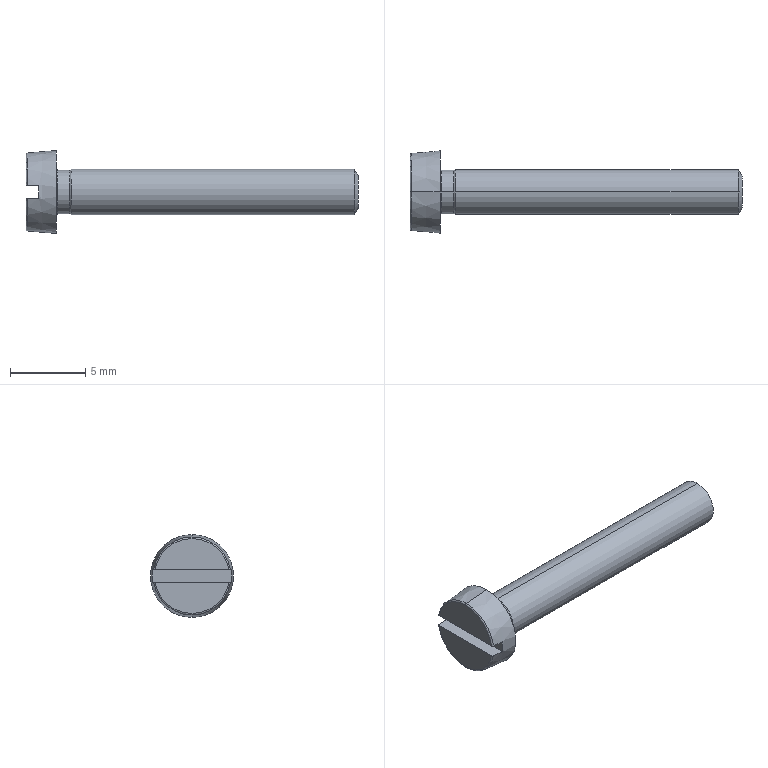Part | SolidWorks | features Cut 1, LPattern 1, RevCut 1, Revolution 1 | 1 solid | 22 faces | box 22 x 5.5 x 5.5 mm | volume 181.48 mm3 | plane 7 | cone 6 | torus 5 | cylinder 4 | commonest cylinder face diameters 2.9 x2 3 x2
STEP:
#1=CARTESIAN_POINT('',(22.,0.,1.067));
#2=VERTEX_POINT('',#1);
#3=CARTESIAN_POINT('',(22.,0.,-1.067));
#4=VERTEX_POINT('',#3);
#5=CARTESIAN_POINT('',(22.,0.,0.));
#6=DIRECTION('',(-1.,0.,0.));
#7=DIRECTION('',(0.,0.,1.));
#8=AXIS2_PLACEMENT_3D('',#5,#6,#7);
#9=CIRCLE('',#8,1.067);
#10=EDGE_CURVE('',#2,#4,#9,.T.);
#11=ORIENTED_EDGE('',*,*,#10,.T.);
#12=CARTESIAN_POINT('',(21.75,0.,-1.5));
#13=VERTEX_POINT('',#12);
#14=CARTESIAN_POINT('',(21.75,0.,-1.5));
#15=DIRECTION('',(-0.5,0.,-0.866));
#16=VECTOR('',#15,1000.);
#17=LINE('',#14,#16);
#18=EDGE_CURVE('',#4,#13,#17,.T.);
#19=ORIENTED_EDGE('',*,*,#18,.T.);
#20=CARTESIAN_POINT('',(21.75,0.,1.5));
#21=VERTEX_POINT('',#20);
#22=CARTESIAN_POINT('',(21.75,0.,0.));
#23=DIRECTION('',(-1.,0.,0.));
#24=DIRECTION('',(0.,0.,1.));
#25=AXIS2_PLACEMENT_3D('',#22,#23,#24);
#26=CIRCLE('',#25,1.5);
#27=EDGE_CURVE('',#21,#13,#26,.T.);
#28=ORIENTED_EDGE('',*,*,#27,.F.);
#29=CARTESIAN_POINT('',(21.75,0.,1.5));
#30=DIRECTION('',(-0.5,0.,0.866));
#31=VECTOR('',#30,1000.);
#32=LINE('',#29,#31);
#33=EDGE_CURVE('',#2,#21,#32,.T.);
#34=ORIENTED_EDGE('',*,*,#33,.F.);
#35=EDGE_LOOP('',(#11,#19,#28,#34));
#36=FACE_OUTER_BOUND('',#35,.T.);
#37=CARTESIAN_POINT('',(21.75,0.,0.));
#38=DIRECTION('',(-1.,0.,0.));
#39=DIRECTION('',(0.,0.,1.));
#40=AXIS2_PLACEMENT_3D('',#37,#38,#39);
#41=CONICAL_SURFACE('',#40,1.5,1.047);
#42=ADVANCED_FACE('',(#36),#41,.T.);
#43=CARTESIAN_POINT('',(2.913,0.,1.45));
#44=VERTEX_POINT('',#43);
#45=CARTESIAN_POINT('',(2.913,0.,-1.45));
#46=VERTEX_POINT('',#45);
#47=CARTESIAN_POINT('',(2.913,0.,0.));
#48=DIRECTION('',(-1.,0.,0.));
#49=DIRECTION('',(0.,0.,1.));
#50=AXIS2_PLACEMENT_3D('',#47,#48,#49);
#51=CIRCLE('',#50,1.45);
#52=EDGE_CURVE('',#44,#46,#51,.T.);
#53=ORIENTED_EDGE('',*,*,#52,.F.);
#54=CARTESIAN_POINT('',(3.,0.,1.5));
#55=VERTEX_POINT('',#54);
#56=CARTESIAN_POINT('',(3.,0.,1.5));
#57=DIRECTION('',(0.866,0.,0.5));
#58=VECTOR('',#57,1000.);
#59=LINE('',#56,#58);
#60=EDGE_CURVE('',#44,#55,#59,.T.);
#61=ORIENTED_EDGE('',*,*,#60,.T.);
#62=CARTESIAN_POINT('',(3.,0.,-1.5));
#63=VERTEX_POINT('',#62);
#64=CARTESIAN_POINT('',(3.,0.,0.));
#65=DIRECTION('',(-1.,0.,0.));
#66=DIRECTION('',(0.,0.,1.));
#67=AXIS2_PLACEMENT_3D('',#64,#65,#66);
#68=CIRCLE('',#67,1.5);
#69=EDGE_CURVE('',#55,#63,#68,.T.);
#70=ORIENTED_EDGE('',*,*,#69,.T.);
#71=CARTESIAN_POINT('',(3.,0.,-1.5));
#72=DIRECTION('',(0.866,0.,-0.5));
#73=VECTOR('',#72,1000.);
#74=LINE('',#71,#73);
#75=EDGE_CURVE('',#46,#63,#74,.T.);
#76=ORIENTED_EDGE('',*,*,#75,.F.);
#77=EDGE_LOOP('',(#53,#61,#70,#76));
#78=FACE_OUTER_BOUND('',#77,.T.);
#79=CARTESIAN_POINT('',(3.,0.,0.));
#80=DIRECTION('',(1.,0.,0.));
#81=DIRECTION('',(0.,0.,-1.));
#82=AXIS2_PLACEMENT_3D('',#79,#80,#81);
#83=CONICAL_SURFACE('',#82,1.5,0.5236);
#84=ADVANCED_FACE('',(#78),#83,.T.);
#85=ORIENTED_EDGE('',*,*,#52,.T.);
#86=CARTESIAN_POINT('',(2.1,0.,-1.45));
#87=VERTEX_POINT('',#86);
#88=CARTESIAN_POINT('',(0.,0.,-1.45));
#89=DIRECTION('',(-1.,0.,0.));
#90=VECTOR('',#89,1000.);
#91=LINE('',#88,#90);
#92=EDGE_CURVE('',#46,#87,#91,.T.);
#93=ORIENTED_EDGE('',*,*,#92,.T.);
#94=CARTESIAN_POINT('',(2.1,0.,1.45));
#95=VERTEX_POINT('',#94);
#96=CARTESIAN_POINT('',(2.1,0.,0.));
#97=DIRECTION('',(-1.,0.,0.));
#98=DIRECTION('',(0.,0.,1.));
#99=AXIS2_PLACEMENT_3D('',#96,#97,#98);
#100=CIRCLE('',#99,1.45);
#101=EDGE_CURVE('',#95,#87,#100,.T.);
#102=ORIENTED_EDGE('',*,*,#101,.F.);
#103=CARTESIAN_POINT('',(0.,0.,1.45));
#104=DIRECTION('',(-1.,0.,0.));
#105=VECTOR('',#104,1000.);
#106=LINE('',#103,#105);
#107=EDGE_CURVE('',#44,#95,#106,.T.);
#108=ORIENTED_EDGE('',*,*,#107,.F.);
#109=EDGE_LOOP('',(#85,#93,#102,#108));
#110=FACE_OUTER_BOUND('',#109,.T.);
#111=CARTESIAN_POINT('',(0.,0.,0.));
#112=DIRECTION('',(-1.,0.,0.));
#113=DIRECTION('',(0.,0.,1.));
#114=AXIS2_PLACEMENT_3D('',#111,#112,#113);
#115=CYLINDRICAL_SURFACE('',#114,1.45);
#116=ADVANCED_FACE('',(#110),#115,.T.);
#117=CARTESIAN_POINT('',(2.,0.,-1.55));
#118=VERTEX_POINT('',#117);
#119=CARTESIAN_POINT('',(2.,0.,1.55));
#120=VERTEX_POINT('',#119);
#121=CARTESIAN_POINT('',(2.,0.,0.));
#122=DIRECTION('',(-1.,0.,0.));
#123=DIRECTION('',(0.,0.,1.));
#124=AXIS2_PLACEMENT_3D('',#121,#122,#123);
#125=CIRCLE('',#124,1.55);
#126=EDGE_CURVE('',#118,#120,#125,.T.);
#127=ORIENTED_EDGE('',*,*,#126,.F.);
#128=CARTESIAN_POINT('',(2.1,0.,-1.55));
#129=DIRECTION('',(0.,1.,0.));
#130=DIRECTION('',(0.,0.,1.));
#131=AXIS2_PLACEMENT_3D('',#128,#129,#130);
#132=CIRCLE('',#131,0.1);
#133=EDGE_CURVE('',#118,#87,#132,.T.);
#134=ORIENTED_EDGE('',*,*,#133,.T.);
#135=CARTESIAN_POINT('',(2.1,0.,0.));
#136=DIRECTION('',(-1.,0.,0.));
#137=DIRECTION('',(0.,0.,1.));
#138=AXIS2_PLACEMENT_3D('',#135,#136,#137);
#139=CIRCLE('',#138,1.45);
#140=EDGE_CURVE('',#87,#95,#139,.T.);
#141=ORIENTED_EDGE('',*,*,#140,.T.);
#142=CARTESIAN_POINT('',(2.1,0.,1.55));
#143=DIRECTION('',(0.,-1.,0.));
#144=DIRECTION('',(0.,0.,-1.));
#145=AXIS2_PLACEMENT_3D('',#142,#143,#144);
#146=CIRCLE('',#145,0.1);
#147=EDGE_CURVE('',#120,#95,#146,.T.);
#148=ORIENTED_EDGE('',*,*,#147,.F.);
#149=EDGE_LOOP('',(#127,#134,#141,#148));
#150=FACE_OUTER_BOUND('',#149,.T.);
#151=CARTESIAN_POINT('',(2.1,0.,0.));
#152=DIRECTION('',(-1.,0.,0.));
#153=DIRECTION('',(0.,0.,1.));
#154=AXIS2_PLACEMENT_3D('',#151,#152,#153);
#155=TOROIDAL_SURFACE('',#154,1.55,0.1);
#156=ADVANCED_FACE('',(#150),#155,.F.);
#157=CARTESIAN_POINT('',(0.09128,0.,2.583));
#158=VERTEX_POINT('',#157);
#159=CARTESIAN_POINT('',(0.09128,2.552,0.4));
#160=VERTEX_POINT('',#159);
#161=CARTESIAN_POINT('',(0.09128,0.,0.));
#162=DIRECTION('',(-1.,0.,0.));
#163=DIRECTION('',(0.,0.,1.));
#164=AXIS2_PLACEMENT_3D('',#161,#162,#163);
#165=CIRCLE('',#164,2.583);
#166=EDGE_CURVE('',#158,#160,#165,.T.);
#167=ORIENTED_EDGE('',*,*,#166,.F.);
#168=CARTESIAN_POINT('',(2.,0.,2.75));
#169=VERTEX_POINT('',#168);
#170=CARTESIAN_POINT('',(2.,0.,2.75));
#171=DIRECTION('',(0.9962,0.,0.08716));
#172=VECTOR('',#171,1000.);
#173=LINE('',#170,#172);
#174=EDGE_CURVE('',#158,#169,#173,.T.);
#175=ORIENTED_EDGE('',*,*,#174,.T.);
#176=CARTESIAN_POINT('',(2.,0.,-2.75));
#177=VERTEX_POINT('',#176);
#178=CARTESIAN_POINT('',(2.,0.,0.));
#179=DIRECTION('',(-1.,0.,0.));
#180=DIRECTION('',(0.,0.,1.));
#181=AXIS2_PLACEMENT_3D('',#178,#179,#180);
#182=CIRCLE('',#181,2.75);
#183=EDGE_CURVE('',#169,#177,#182,.T.);
#184=ORIENTED_EDGE('',*,*,#183,.T.);
#185=CARTESIAN_POINT('',(0.09128,0.,-2.583));
#186=VERTEX_POINT('',#185);
#187=CARTESIAN_POINT('',(2.,0.,-2.75));
#188=DIRECTION('',(0.9962,0.,-0.08716));
#189=VECTOR('',#188,1000.);
#190=LINE('',#187,#189);
#191=EDGE_CURVE('',#186,#177,#190,.T.);
#192=ORIENTED_EDGE('',*,*,#191,.F.);
#193=CARTESIAN_POINT('',(0.09128,2.552,-0.4));
#194=VERTEX_POINT('',#193);
#195=CARTESIAN_POINT('',(0.09128,0.,0.));
#196=DIRECTION('',(-1.,0.,0.));
#197=DIRECTION('',(0.,0.,1.));
#198=AXIS2_PLACEMENT_3D('',#195,#196,#197);
#199=CIRCLE('',#198,2.583);
#200=EDGE_CURVE('',#194,#186,#199,.T.);
#201=ORIENTED_EDGE('',*,*,#200,.F.);
#202=CARTESIAN_POINT('',(0.85,2.619,-0.4));
#203=VERTEX_POINT('',#202);
#204=CARTESIAN_POINT('',(0.09128,2.552,-0.4));
#205=CARTESIAN_POINT('',(0.2017,2.562,-0.4));
#206=CARTESIAN_POINT('',(0.3121,2.571,-0.4));
#207=CARTESIAN_POINT('',(0.4225,2.581,-0.4));
#208=CARTESIAN_POINT('',(0.565,2.594,-0.4));
#209=CARTESIAN_POINT('',(0.7075,2.606,-0.4));
#210=CARTESIAN_POINT('',(0.85,2.619,-0.4));
#211=B_SPLINE_CURVE_WITH_KNOTS('',3,(#204,#205,#206,#207,#208,#209,#210),.UNSPECIFIED.,.F.,.F.,(4,3,4),(0.004473,0.004805,0.005234),.UNSPECIFIED.);
#212=EDGE_CURVE('',#194,#203,#211,.T.);
#213=ORIENTED_EDGE('',*,*,#212,.T.);
#214=CARTESIAN_POINT('',(0.85,2.619,0.4));
#215=VERTEX_POINT('',#214);
#216=CARTESIAN_POINT('',(0.85,0.,0.));
#217=DIRECTION('',(-1.,0.,0.));
#218=DIRECTION('',(0.,-1.,0.));
#219=AXIS2_PLACEMENT_3D('',#216,#217,#218);
#220=CIRCLE('',#219,2.649);
#221=EDGE_CURVE('',#215,#203,#220,.T.);
#222=ORIENTED_EDGE('',*,*,#221,.F.);
#223=CARTESIAN_POINT('',(0.85,2.619,0.4));
#224=CARTESIAN_POINT('',(0.7075,2.606,0.4));
#225=CARTESIAN_POINT('',(0.565,2.594,0.4));
#226=CARTESIAN_POINT('',(0.4225,2.581,0.4));
#227=CARTESIAN_POINT('',(0.3121,2.571,0.4));
#228=CARTESIAN_POINT('',(0.2017,2.562,0.4));
#229=CARTESIAN_POINT('',(0.09128,2.552,0.4));
#230=B_SPLINE_CURVE_WITH_KNOTS('',3,(#223,#224,#225,#226,#227,#228,#229),.UNSPECIFIED.,.F.,.F.,(4,3,4),(0.004376,0.004805,0.005138),.UNSPECIFIED.);
#231=EDGE_CURVE('',#215,#160,#230,.T.);
#232=ORIENTED_EDGE('',*,*,#231,.T.);
#233=EDGE_LOOP('',(#167,#175,#184,#192,#201,#213,#222,#232));
#234=FACE_OUTER_BOUND('',#233,.T.);
#235=CARTESIAN_POINT('',(2.,0.,0.));
#236=DIRECTION('',(1.,0.,0.));
#237=DIRECTION('',(0.,0.,-1.));
#238=AXIS2_PLACEMENT_3D('',#235,#236,#237);
#239=CONICAL_SURFACE('',#238,2.75,0.08727);
#240=ADVANCED_FACE('',(#234),#239,.T.);
#241=CARTESIAN_POINT('',(0.09128,-2.552,0.4));
#242=VERTEX_POINT('',#241);
#243=CARTESIAN_POINT('',(0.09128,0.,0.));
#244=DIRECTION('',(-1.,0.,0.));
#245=DIRECTION('',(0.,0.,1.));
#246=AXIS2_PLACEMENT_3D('',#243,#244,#245);
#247=CIRCLE('',#246,2.583);
#248=EDGE_CURVE('',#242,#158,#247,.T.);
#249=ORIENTED_EDGE('',*,*,#248,.T.);
#250=CARTESIAN_POINT('',(0.,0.,2.483));
#251=VERTEX_POINT('',#250);
#252=CARTESIAN_POINT('',(0.1,0.,2.483));
#253=DIRECTION('',(0.,-1.,0.));
#254=DIRECTION('',(0.,0.,-1.));
#255=AXIS2_PLACEMENT_3D('',#252,#253,#254);
#256=CIRCLE('',#255,0.1);
#257=EDGE_CURVE('',#158,#251,#256,.T.);
#258=ORIENTED_EDGE('',*,*,#257,.T.);
#259=CARTESIAN_POINT('',(0.,-2.451,0.4));
#260=VERTEX_POINT('',#259);
#261=CARTESIAN_POINT('',(0.,0.,0.));
#262=DIRECTION('',(-1.,0.,0.));
#263=DIRECTION('',(0.,0.,1.));
#264=AXIS2_PLACEMENT_3D('',#261,#262,#263);
#265=CIRCLE('',#264,2.483);
#266=EDGE_CURVE('',#260,#251,#265,.T.);
#267=ORIENTED_EDGE('',*,*,#266,.F.);
#268=CARTESIAN_POINT('',(0.,-2.451,0.4));
#269=CARTESIAN_POINT('',(0.,-2.458,0.4));
#270=CARTESIAN_POINT('',(0.0008068,-2.466,0.4));
#271=CARTESIAN_POINT('',(0.002394,-2.473,0.4));
#272=CARTESIAN_POINT('',(0.004862,-2.484,0.4));
#273=CARTESIAN_POINT('',(0.009305,-2.495,0.4));
#274=CARTESIAN_POINT('',(0.01537,-2.505,0.4));
#275=CARTESIAN_POINT('',(0.01925,-2.511,0.4));
#276=CARTESIAN_POINT('',(0.02385,-2.517,0.4));
#277=CARTESIAN_POINT('',(0.02899,-2.522,0.4));
#278=CARTESIAN_POINT('',(0.03681,-2.53,0.4));
#279=CARTESIAN_POINT('',(0.04609,-2.537,0.4));
#280=CARTESIAN_POINT('',(0.0561,-2.542,0.4));
#281=CARTESIAN_POINT('',(0.06611,-2.547,0.4));
#282=CARTESIAN_POINT('',(0.07712,-2.55,0.4));
#283=CARTESIAN_POINT('',(0.0882,-2.552,0.4));
#284=CARTESIAN_POINT('',(0.08923,-2.552,0.4));
#285=CARTESIAN_POINT('',(0.09026,-2.552,0.4));
#286=CARTESIAN_POINT('',(0.09128,-2.552,0.4));
#287=B_SPLINE_CURVE_WITH_KNOTS('',3,(#268,#269,#270,#271,#272,#273,#274,#275,#276,#277,#278,#279,#280,#281,#282,#283,#284,#285,#286),.UNSPECIFIED.,.F.,.F.,(4,3,3,3,3,3,4),(0.0005509,0.0005731,0.0006075,0.0006294,0.0006629,0.0006964,0.0006995),.UNSPECIFIED.);
#288=EDGE_CURVE('',#260,#242,#287,.T.);
#289=ORIENTED_EDGE('',*,*,#288,.T.);
#290=EDGE_LOOP('',(#249,#258,#267,#289));
#291=FACE_OUTER_BOUND('',#290,.T.);
#292=CARTESIAN_POINT('',(0.1,0.,0.));
#293=DIRECTION('',(-1.,0.,0.));
#294=DIRECTION('',(0.,0.,1.));
#295=AXIS2_PLACEMENT_3D('',#292,#293,#294);
#296=TOROIDAL_SURFACE('',#295,2.483,0.1);
#297=ADVANCED_FACE('',(#291),#296,.T.);
#298=ORIENTED_EDGE('',*,*,#27,.T.);
#299=CARTESIAN_POINT('',(0.,0.,-1.5));
#300=DIRECTION('',(-1.,0.,0.));
#301=VECTOR('',#300,1000.);
#302=LINE('',#299,#301);
#303=EDGE_CURVE('',#13,#63,#302,.T.);
#304=ORIENTED_EDGE('',*,*,#303,.T.);
#305=ORIENTED_EDGE('',*,*,#69,.F.);
#306=CARTESIAN_POINT('',(0.,0.,1.5));
#307=DIRECTION('',(-1.,0.,0.));
#308=VECTOR('',#307,1000.);
#309=LINE('',#306,#308);
#310=EDGE_CURVE('',#21,#55,#309,.T.);
#311=ORIENTED_EDGE('',*,*,#310,.F.);
#312=EDGE_LOOP('',(#298,#304,#305,#311));
#313=FACE_OUTER_BOUND('',#312,.T.);
#314=CARTESIAN_POINT('',(0.,0.,0.));
#315=DIRECTION('',(-1.,0.,0.));
#316=DIRECTION('',(0.,0.,1.));
#317=AXIS2_PLACEMENT_3D('',#314,#315,#316);
#318=CYLINDRICAL_SURFACE('',#317,1.5);
#319=ADVANCED_FACE('',(#313),#318,.T.);
#320=ORIENTED_EDGE('',*,*,#303,.F.);
#321=CARTESIAN_POINT('',(21.75,0.,0.));
#322=DIRECTION('',(-1.,0.,0.));
#323=DIRECTION('',(0.,0.,1.));
#324=AXIS2_PLACEMENT_3D('',#321,#322,#323);
#325=CIRCLE('',#324,1.5);
#326=EDGE_CURVE('',#13,#21,#325,.T.);
#327=ORIENTED_EDGE('',*,*,#326,.T.);
#328=ORIENTED_EDGE('',*,*,#310,.T.);
#329=CARTESIAN_POINT('',(3.,0.,0.));
#330=DIRECTION('',(-1.,0.,0.));
#331=DIRECTION('',(0.,0.,1.));
#332=AXIS2_PLACEMENT_3D('',#329,#330,#331);
#333=CIRCLE('',#332,1.5);
#334=EDGE_CURVE('',#63,#55,#333,.T.);
#335=ORIENTED_EDGE('',*,*,#334,.F.);
#336=EDGE_LOOP('',(#320,#327,#328,#335));
#337=FACE_OUTER_BOUND('',#336,.T.);
#338=CARTESIAN_POINT('',(0.,0.,0.));
#339=DIRECTION('',(-1.,0.,0.));
#340=DIRECTION('',(0.,0.,1.));
#341=AXIS2_PLACEMENT_3D('',#338,#339,#340);
#342=CYLINDRICAL_SURFACE('',#341,1.5);
#343=ADVANCED_FACE('',(#337),#342,.T.);
#344=ORIENTED_EDGE('',*,*,#266,.T.);
#345=CARTESIAN_POINT('',(0.,2.451,0.4));
#346=VERTEX_POINT('',#345);
#347=CARTESIAN_POINT('',(0.,0.,0.));
#348=DIRECTION('',(-1.,0.,0.));
#349=DIRECTION('',(0.,0.,1.));
#350=AXIS2_PLACEMENT_3D('',#347,#348,#349);
#351=CIRCLE('',#350,2.483);
#352=EDGE_CURVE('',#251,#346,#351,.T.);
#353=ORIENTED_EDGE('',*,*,#352,.T.);
#354=CARTESIAN_POINT('',(0.,2.721,0.4));
#355=DIRECTION('',(0.,1.,0.));
#356=VECTOR('',#355,1000.);
#357=LINE('',#354,#356);
#358=EDGE_CURVE('',#260,#346,#357,.T.);
#359=ORIENTED_EDGE('',*,*,#358,.F.);
#360=EDGE_LOOP('',(#344,#353,#359));
#361=FACE_OUTER_BOUND('',#360,.T.);
#362=CARTESIAN_POINT('',(0.,0.,0.));
#363=DIRECTION('',(1.,0.,0.));
#364=DIRECTION('',(0.,0.,-1.));
#365=AXIS2_PLACEMENT_3D('',#362,#363,#364);
#366=PLANE('',#365);
#367=ADVANCED_FACE('',(#361),#366,.F.);
#368=ORIENTED_EDGE('',*,*,#257,.F.);
#369=ORIENTED_EDGE('',*,*,#166,.T.);
#370=CARTESIAN_POINT('',(0.09128,2.552,0.4));
#371=CARTESIAN_POINT('',(0.08707,2.551,0.4));
#372=CARTESIAN_POINT('',(0.08288,2.551,0.4));
#373=CARTESIAN_POINT('',(0.07875,2.55,0.4));
#374=CARTESIAN_POINT('',(0.06795,2.548,0.4));
#375=CARTESIAN_POINT('',(0.05741,2.543,0.4));
#376=CARTESIAN_POINT('',(0.048,2.537,0.4));
#377=CARTESIAN_POINT('',(0.03854,2.532,0.4));
#378=CARTESIAN_POINT('',(0.02995,2.524,0.4));
#379=CARTESIAN_POINT('',(0.02293,2.516,0.4));
#380=CARTESIAN_POINT('',(0.01583,2.507,0.4));
#381=CARTESIAN_POINT('',(0.01012,2.497,0.4));
#382=CARTESIAN_POINT('',(0.006257,2.486,0.4));
#383=CARTESIAN_POINT('',(0.002345,2.476,0.4));
#384=CARTESIAN_POINT('',(0.0002101,2.464,0.4));
#385=CARTESIAN_POINT('',(0.00001512,2.453,0.4));
#386=CARTESIAN_POINT('',(0.00000504,2.452,0.4));
#387=CARTESIAN_POINT('',(0.,2.452,0.4));
#388=CARTESIAN_POINT('',(0.,2.451,0.4));
#389=B_SPLINE_CURVE_WITH_KNOTS('',3,(#370,#371,#372,#373,#374,#375,#376,#377,#378,#379,#380,#381,#382,#383,#384,#385,#386,#387,#388),.UNSPECIFIED.,.F.,.F.,(4,3,3,3,3,3,4),(0.0003918,0.0004044,0.0004376,0.0004709,0.0005046,0.0005387,0.0005404),.UNSPECIFIED.);
#390=EDGE_CURVE('',#160,#346,#389,.T.);
#391=ORIENTED_EDGE('',*,*,#390,.T.);
#392=ORIENTED_EDGE('',*,*,#352,.F.);
#393=EDGE_LOOP('',(#368,#369,#391,#392));
#394=FACE_OUTER_BOUND('',#393,.T.);
#395=CARTESIAN_POINT('',(0.1,0.,0.));
#396=DIRECTION('',(-1.,0.,0.));
#397=DIRECTION('',(0.,0.,1.));
#398=AXIS2_PLACEMENT_3D('',#395,#396,#397);
#399=TOROIDAL_SURFACE('',#398,2.483,0.1);
#400=ADVANCED_FACE('',(#394),#399,.T.);
#401=CARTESIAN_POINT('',(0.,2.451,-0.4));
#402=VERTEX_POINT('',#401);
#403=CARTESIAN_POINT('',(0.,-2.451,-0.4));
#404=VERTEX_POINT('',#403);
#405=CARTESIAN_POINT('',(0.,0.,0.));
#406=DIRECTION('',(-1.,0.,0.));
#407=DIRECTION('',(0.,0.,1.));
#408=AXIS2_PLACEMENT_3D('',#405,#406,#407);
#409=CIRCLE('',#408,2.483);
#410=EDGE_CURVE('',#402,#404,#409,.T.);
#411=ORIENTED_EDGE('',*,*,#410,.T.);
#412=CARTESIAN_POINT('',(0.,2.721,-0.4));
#413=DIRECTION('',(0.,-1.,0.));
#414=VECTOR('',#413,1000.);
#415=LINE('',#412,#414);
#416=EDGE_CURVE('',#402,#404,#415,.T.);
#417=ORIENTED_EDGE('',*,*,#416,.F.);
#418=EDGE_LOOP('',(#411,#417));
#419=FACE_OUTER_BOUND('',#418,.T.);
#420=CARTESIAN_POINT('',(0.,0.,0.));
#421=DIRECTION('',(1.,0.,0.));
#422=DIRECTION('',(0.,0.,-1.));
#423=AXIS2_PLACEMENT_3D('',#420,#421,#422);
#424=PLANE('',#423);
#425=ADVANCED_FACE('',(#419),#424,.F.);
#426=ORIENTED_EDGE('',*,*,#200,.T.);
#427=CARTESIAN_POINT('',(0.09128,-2.552,-0.4));
#428=VERTEX_POINT('',#427);
#429=CARTESIAN_POINT('',(0.09128,0.,0.));
#430=DIRECTION('',(-1.,0.,0.));
#431=DIRECTION('',(0.,0.,1.));
#432=AXIS2_PLACEMENT_3D('',#429,#430,#431);
#433=CIRCLE('',#432,2.583);
#434=EDGE_CURVE('',#186,#428,#433,.T.);
#435=ORIENTED_EDGE('',*,*,#434,.T.);
#436=CARTESIAN_POINT('',(0.09128,-2.552,-0.4));
#437=CARTESIAN_POINT('',(0.08571,-2.551,-0.4));
#438=CARTESIAN_POINT('',(0.08015,-2.55,-0.4));
#439=CARTESIAN_POINT('',(0.07474,-2.549,-0.4));
#440=CARTESIAN_POINT('',(0.06404,-2.546,-0.4));
#441=CARTESIAN_POINT('',(0.05369,-2.541,-0.4));
#442=CARTESIAN_POINT('',(0.04452,-2.535,-0.4));
#443=CARTESIAN_POINT('',(0.03893,-2.531,-0.4));
#444=CARTESIAN_POINT('',(0.03371,-2.527,-0.4));
#445=CARTESIAN_POINT('',(0.02899,-2.522,-0.4));
#446=CARTESIAN_POINT('',(0.02104,-2.514,-0.4));
#447=CARTESIAN_POINT('',(0.0144,-2.505,-0.4));
#448=CARTESIAN_POINT('',(0.009591,-2.494,-0.4));
#449=CARTESIAN_POINT('',(0.004787,-2.484,-0.4));
#450=CARTESIAN_POINT('',(0.001687,-2.473,-0.4));
#451=CARTESIAN_POINT('',(0.0005321,-2.461,-0.4));
#452=CARTESIAN_POINT('',(0.0001778,-2.458,-0.4));
#453=CARTESIAN_POINT('',(0.,-2.454,-0.4));
#454=CARTESIAN_POINT('',(0.,-2.451,-0.4));
#455=B_SPLINE_CURVE_WITH_KNOTS('',3,(#436,#437,#438,#439,#440,#441,#442,#443,#444,#445,#446,#447,#448,#449,#450,#451,#452,#453,#454),.UNSPECIFIED.,.F.,.F.,(4,3,3,3,3,3,4),(0.0005594,0.0005761,0.0006093,0.0006293,0.0006634,0.0006975,0.0007078),.UNSPECIFIED.);
#456=EDGE_CURVE('',#428,#404,#455,.T.);
#457=ORIENTED_EDGE('',*,*,#456,.T.);
#458=ORIENTED_EDGE('',*,*,#410,.F.);
#459=CARTESIAN_POINT('',(0.,2.451,-0.4));
#460=CARTESIAN_POINT('',(0.,2.455,-0.4));
#461=CARTESIAN_POINT('',(0.000287,2.46,-0.4));
#462=CARTESIAN_POINT('',(0.0008577,2.464,-0.4));
#463=CARTESIAN_POINT('',(0.00234,2.476,-0.4));
#464=CARTESIAN_POINT('',(0.005811,2.487,-0.4));
#465=CARTESIAN_POINT('',(0.011,2.497,-0.4));
#466=CARTESIAN_POINT('',(0.01616,2.507,-0.4));
#467=CARTESIAN_POINT('',(0.02317,2.517,-0.4));
#468=CARTESIAN_POINT('',(0.03145,2.525,-0.4));
#469=CARTESIAN_POINT('',(0.03965,2.533,-0.4));
#470=CARTESIAN_POINT('',(0.04932,2.539,-0.4));
#471=CARTESIAN_POINT('',(0.05966,2.544,-0.4));
#472=CARTESIAN_POINT('',(0.0696,2.548,-0.4));
#473=CARTESIAN_POINT('',(0.08043,2.551,-0.4));
#474=CARTESIAN_POINT('',(0.09128,2.552,-0.4));
#475=B_SPLINE_CURVE_WITH_KNOTS('',3,(#459,#460,#461,#462,#463,#464,#465,#466,#467,#468,#469,#470,#471,#472,#473,#474),.UNSPECIFIED.,.F.,.F.,(4,3,3,3,3,4),(0.00008915,0.0001023,0.0001368,0.0001712,0.0002051,0.0002378),.UNSPECIFIED.);
#476=EDGE_CURVE('',#402,#194,#475,.T.);
#477=ORIENTED_EDGE('',*,*,#476,.T.);
#478=EDGE_LOOP('',(#426,#435,#457,#458,#477));
#479=FACE_OUTER_BOUND('',#478,.T.);
#480=CARTESIAN_POINT('',(0.1,0.,0.));
#481=DIRECTION('',(-1.,0.,0.));
#482=DIRECTION('',(0.,0.,1.));
#483=AXIS2_PLACEMENT_3D('',#480,#481,#482);
#484=TOROIDAL_SURFACE('',#483,2.483,0.1);
#485=ADVANCED_FACE('',(#479),#484,.T.);
#486=ORIENTED_EDGE('',*,*,#174,.F.);
#487=ORIENTED_EDGE('',*,*,#248,.F.);
#488=CARTESIAN_POINT('',(0.85,-2.619,0.4));
#489=VERTEX_POINT('',#488);
#490=CARTESIAN_POINT('',(0.09128,-2.552,0.4));
#491=CARTESIAN_POINT('',(0.2017,-2.562,0.4));
#492=CARTESIAN_POINT('',(0.3121,-2.571,0.4));
#493=CARTESIAN_POINT('',(0.4225,-2.581,0.4));
#494=CARTESIAN_POINT('',(0.565,-2.594,0.4));
#495=CARTESIAN_POINT('',(0.7075,-2.606,0.4));
#496=CARTESIAN_POINT('',(0.85,-2.619,0.4));
#497=B_SPLINE_CURVE_WITH_KNOTS('',3,(#490,#491,#492,#493,#494,#495,#496),.UNSPECIFIED.,.F.,.F.,(4,3,4),(0.004473,0.004805,0.005234),.UNSPECIFIED.);
#498=EDGE_CURVE('',#242,#489,#497,.T.);
#499=ORIENTED_EDGE('',*,*,#498,.T.);
#500=CARTESIAN_POINT('',(0.85,-2.619,-0.4));
#501=VERTEX_POINT('',#500);
#502=CARTESIAN_POINT('',(0.85,0.,0.));
#503=DIRECTION('',(-1.,0.,0.));
#504=DIRECTION('',(0.,-1.,0.));
#505=AXIS2_PLACEMENT_3D('',#502,#503,#504);
#506=CIRCLE('',#505,2.649);
#507=EDGE_CURVE('',#501,#489,#506,.T.);
#508=ORIENTED_EDGE('',*,*,#507,.F.);
#509=CARTESIAN_POINT('',(0.85,-2.619,-0.4));
#510=CARTESIAN_POINT('',(0.7075,-2.606,-0.4));
#511=CARTESIAN_POINT('',(0.565,-2.594,-0.4));
#512=CARTESIAN_POINT('',(0.4225,-2.581,-0.4));
#513=CARTESIAN_POINT('',(0.3121,-2.571,-0.4));
#514=CARTESIAN_POINT('',(0.2017,-2.562,-0.4));
#515=CARTESIAN_POINT('',(0.09128,-2.552,-0.4));
#516=B_SPLINE_CURVE_WITH_KNOTS('',3,(#509,#510,#511,#512,#513,#514,#515),.UNSPECIFIED.,.F.,.F.,(4,3,4),(0.004376,0.004805,0.005138),.UNSPECIFIED.);
#517=EDGE_CURVE('',#501,#428,#516,.T.);
#518=ORIENTED_EDGE('',*,*,#517,.T.);
#519=ORIENTED_EDGE('',*,*,#434,.F.);
#520=ORIENTED_EDGE('',*,*,#191,.T.);
#521=CARTESIAN_POINT('',(2.,0.,0.));
#522=DIRECTION('',(-1.,0.,0.));
#523=DIRECTION('',(0.,0.,1.));
#524=AXIS2_PLACEMENT_3D('',#521,#522,#523);
#525=CIRCLE('',#524,2.75);
#526=EDGE_CURVE('',#177,#169,#525,.T.);
#527=ORIENTED_EDGE('',*,*,#526,.T.);
#528=EDGE_LOOP('',(#486,#487,#499,#508,#518,#519,#520,#527));
#529=FACE_OUTER_BOUND('',#528,.T.);
#530=CARTESIAN_POINT('',(2.,0.,0.));
#531=DIRECTION('',(1.,0.,0.));
#532=DIRECTION('',(0.,0.,-1.));
#533=AXIS2_PLACEMENT_3D('',#530,#531,#532);
#534=CONICAL_SURFACE('',#533,2.75,0.08727);
#535=ADVANCED_FACE('',(#529),#534,.T.);
#536=ORIENTED_EDGE('',*,*,#526,.F.);
#537=ORIENTED_EDGE('',*,*,#183,.F.);
#538=EDGE_LOOP('',(#536,#537));
#539=FACE_OUTER_BOUND('',#538,.T.);
#540=CARTESIAN_POINT('',(2.,0.,0.));
#541=DIRECTION('',(-1.,0.,0.));
#542=DIRECTION('',(0.,0.,1.));
#543=AXIS2_PLACEMENT_3D('',#540,#541,#542);
#544=CIRCLE('',#543,1.55);
#545=EDGE_CURVE('',#120,#118,#544,.T.);
#546=ORIENTED_EDGE('',*,*,#545,.T.);
#547=ORIENTED_EDGE('',*,*,#126,.T.);
#548=EDGE_LOOP('',(#546,#547));
#549=FACE_BOUND('',#548,.T.);
#550=CARTESIAN_POINT('',(2.,2.75,0.));
#551=DIRECTION('',(-1.,0.,0.));
#552=DIRECTION('',(0.,0.,1.));
#553=AXIS2_PLACEMENT_3D('',#550,#551,#552);
#554=PLANE('',#553);
#555=ADVANCED_FACE('',(#539,#549),#554,.F.);
#556=ORIENTED_EDGE('',*,*,#133,.F.);
#557=ORIENTED_EDGE('',*,*,#545,.F.);
#558=ORIENTED_EDGE('',*,*,#147,.T.);
#559=ORIENTED_EDGE('',*,*,#101,.T.);
#560=EDGE_LOOP('',(#556,#557,#558,#559));
#561=FACE_OUTER_BOUND('',#560,.T.);
#562=CARTESIAN_POINT('',(2.1,0.,0.));
#563=DIRECTION('',(-1.,0.,0.));
#564=DIRECTION('',(0.,0.,1.));
#565=AXIS2_PLACEMENT_3D('',#562,#563,#564);
#566=TOROIDAL_SURFACE('',#565,1.55,0.1);
#567=ADVANCED_FACE('',(#561),#566,.F.);
#568=ORIENTED_EDGE('',*,*,#92,.F.);
#569=CARTESIAN_POINT('',(2.913,0.,0.));
#570=DIRECTION('',(-1.,0.,0.));
#571=DIRECTION('',(0.,0.,1.));
#572=AXIS2_PLACEMENT_3D('',#569,#570,#571);
#573=CIRCLE('',#572,1.45);
#574=EDGE_CURVE('',#46,#44,#573,.T.);
#575=ORIENTED_EDGE('',*,*,#574,.T.);
#576=ORIENTED_EDGE('',*,*,#107,.T.);
#577=ORIENTED_EDGE('',*,*,#140,.F.);
#578=EDGE_LOOP('',(#568,#575,#576,#577));
#579=FACE_OUTER_BOUND('',#578,.T.);
#580=CARTESIAN_POINT('',(0.,0.,0.));
#581=DIRECTION('',(-1.,0.,0.));
#582=DIRECTION('',(0.,0.,1.));
#583=AXIS2_PLACEMENT_3D('',#580,#581,#582);
#584=CYLINDRICAL_SURFACE('',#583,1.45);
#585=ADVANCED_FACE('',(#579),#584,.T.);
#586=ORIENTED_EDGE('',*,*,#60,.F.);
#587=ORIENTED_EDGE('',*,*,#574,.F.);
#588=ORIENTED_EDGE('',*,*,#75,.T.);
#589=ORIENTED_EDGE('',*,*,#334,.T.);
#590=EDGE_LOOP('',(#586,#587,#588,#589));
#591=FACE_OUTER_BOUND('',#590,.T.);
#592=CARTESIAN_POINT('',(3.,0.,0.));
#593=DIRECTION('',(1.,0.,0.));
#594=DIRECTION('',(0.,0.,-1.));
#595=AXIS2_PLACEMENT_3D('',#592,#593,#594);
#596=CONICAL_SURFACE('',#595,1.5,0.5236);
#597=ADVANCED_FACE('',(#591),#596,.T.);
#598=ORIENTED_EDGE('',*,*,#358,.T.);
#599=ORIENTED_EDGE('',*,*,#390,.F.);
#600=ORIENTED_EDGE('',*,*,#231,.F.);
#601=CARTESIAN_POINT('',(0.85,2.721,0.4));
#602=DIRECTION('',(0.,1.,0.));
#603=VECTOR('',#602,1000.);
#604=LINE('',#601,#603);
#605=EDGE_CURVE('',#489,#215,#604,.T.);
#606=ORIENTED_EDGE('',*,*,#605,.F.);
#607=ORIENTED_EDGE('',*,*,#498,.F.);
#608=ORIENTED_EDGE('',*,*,#288,.F.);
#609=EDGE_LOOP('',(#598,#599,#600,#606,#607,#608));
#610=FACE_OUTER_BOUND('',#609,.T.);
#611=CARTESIAN_POINT('',(0.85,2.721,0.4));
#612=DIRECTION('',(0.,0.,1.));
#613=DIRECTION('',(0.,-1.,0.));
#614=AXIS2_PLACEMENT_3D('',#611,#612,#613);
#615=PLANE('',#614);
#616=ADVANCED_FACE('',(#610),#615,.F.);
#617=ORIENTED_EDGE('',*,*,#517,.F.);
#618=CARTESIAN_POINT('',(0.85,2.721,-0.4));
#619=DIRECTION('',(0.,-1.,0.));
#620=VECTOR('',#619,1000.);
#621=LINE('',#618,#620);
#622=EDGE_CURVE('',#203,#501,#621,.T.);
#623=ORIENTED_EDGE('',*,*,#622,.F.);
#624=ORIENTED_EDGE('',*,*,#212,.F.);
#625=ORIENTED_EDGE('',*,*,#476,.F.);
#626=ORIENTED_EDGE('',*,*,#416,.T.);
#627=ORIENTED_EDGE('',*,*,#456,.F.);
#628=EDGE_LOOP('',(#617,#623,#624,#625,#626,#627));
#629=FACE_OUTER_BOUND('',#628,.T.);
#630=CARTESIAN_POINT('',(0.85,2.721,-0.4));
#631=DIRECTION('',(0.,0.,-1.));
#632=DIRECTION('',(-1.,0.,0.));
#633=AXIS2_PLACEMENT_3D('',#630,#631,#632);
#634=PLANE('',#633);
#635=ADVANCED_FACE('',(#629),#634,.F.);
#636=ORIENTED_EDGE('',*,*,#221,.T.);
#637=ORIENTED_EDGE('',*,*,#622,.T.);
#638=ORIENTED_EDGE('',*,*,#507,.T.);
#639=ORIENTED_EDGE('',*,*,#605,.T.);
#640=EDGE_LOOP('',(#636,#637,#638,#639));
#641=FACE_OUTER_BOUND('',#640,.T.);
#642=CARTESIAN_POINT('',(0.85,0.,0.));
#643=DIRECTION('',(-1.,0.,0.));
#644=DIRECTION('',(0.,-1.,0.));
#645=AXIS2_PLACEMENT_3D('',#642,#643,#644);
#646=PLANE('',#645);
#647=ADVANCED_FACE('',(#641),#646,.T.);
#648=ORIENTED_EDGE('',*,*,#18,.F.);
#649=CARTESIAN_POINT('',(22.,0.,0.));
#650=DIRECTION('',(-1.,0.,0.));
#651=DIRECTION('',(0.,0.,1.));
#652=AXIS2_PLACEMENT_3D('',#649,#650,#651);
#653=CIRCLE('',#652,1.067);
#654=EDGE_CURVE('',#4,#2,#653,.T.);
#655=ORIENTED_EDGE('',*,*,#654,.T.);
#656=ORIENTED_EDGE('',*,*,#33,.T.);
#657=ORIENTED_EDGE('',*,*,#326,.F.);
#658=EDGE_LOOP('',(#648,#655,#656,#657));
#659=FACE_OUTER_BOUND('',#658,.T.);
#660=CARTESIAN_POINT('',(21.75,0.,0.));
#661=DIRECTION('',(-1.,0.,0.));
#662=DIRECTION('',(0.,0.,1.));
#663=AXIS2_PLACEMENT_3D('',#660,#661,#662);
#664=CONICAL_SURFACE('',#663,1.5,1.047);
#665=ADVANCED_FACE('',(#659),#664,.T.);
#666=ORIENTED_EDGE('',*,*,#10,.F.);
#667=ORIENTED_EDGE('',*,*,#654,.F.);
#668=EDGE_LOOP('',(#666,#667));
#669=FACE_OUTER_BOUND('',#668,.T.);
#670=CARTESIAN_POINT('',(22.,1.5,0.));
#671=DIRECTION('',(-1.,0.,0.));
#672=DIRECTION('',(0.,0.,1.));
#673=AXIS2_PLACEMENT_3D('',#670,#671,#672);
#674=PLANE('',#673);
#675=ADVANCED_FACE('',(#669),#674,.F.);
#676=CLOSED_SHELL('',(#42,#84,#116,#156,#240,#297,#319,#343,#367,#400,#425,#485,#535,#555,#567,#585,#597,#616,#635,#647,#665,#675));
#677=MANIFOLD_SOLID_BREP('',#676);
#678=CARTESIAN_POINT('',(0.,0.,0.));
#679=DIRECTION('',(0.,0.,1.));
#680=DIRECTION('',(1.,0.,0.));
#681=AXIS2_PLACEMENT_3D('',#678,#679,#680);
#682=(LENGTH_UNIT()NAMED_UNIT(*)SI_UNIT(.MILLI.,.METRE.));
#683=UNCERTAINTY_MEASURE_WITH_UNIT(LENGTH_MEASURE(0.00001),#682,'','');
#684=(NAMED_UNIT(*)PLANE_ANGLE_UNIT()SI_UNIT($,.RADIAN.));
#685=(NAMED_UNIT(*)SI_UNIT($,.STERADIAN.)SOLID_ANGLE_UNIT());
#686=(GEOMETRIC_REPRESENTATION_CONTEXT(3)GLOBAL_UNCERTAINTY_ASSIGNED_CONTEXT((#683))GLOBAL_UNIT_ASSIGNED_CONTEXT((#682,#684,#685))REPRESENTATION_CONTEXT('',''));
#687=ADVANCED_BREP_SHAPE_REPRESENTATION('',(#677,#681),#686);